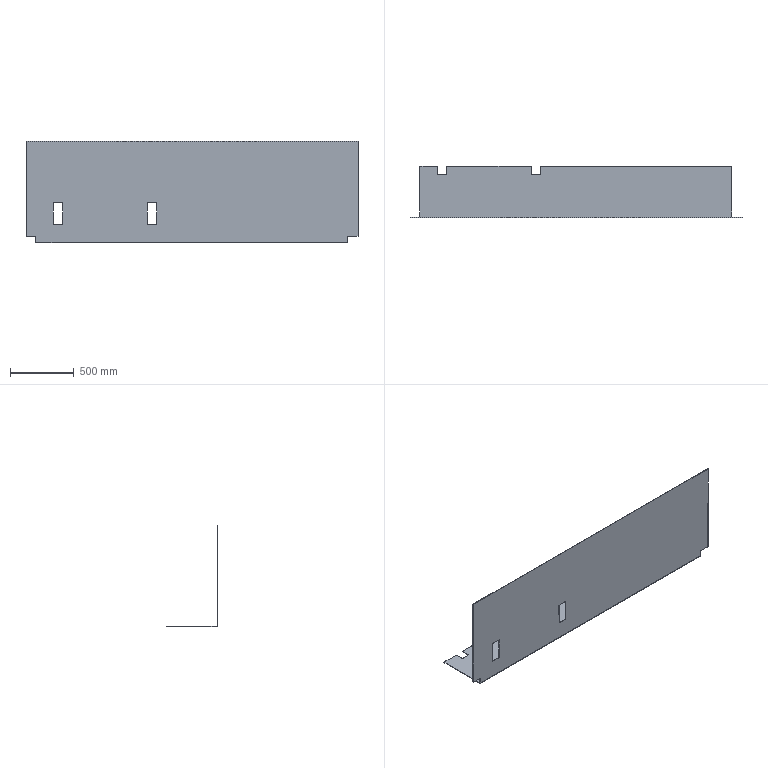Part | STEP file | E3-花纹Plate折弯4 | 1 solid | 30 faces | box 2600 x 403 x 798 mm | volume 12012783 mm3 | plane 28 | cylinder 2 | commonest cylinder face diameters 2 x1 10 x1